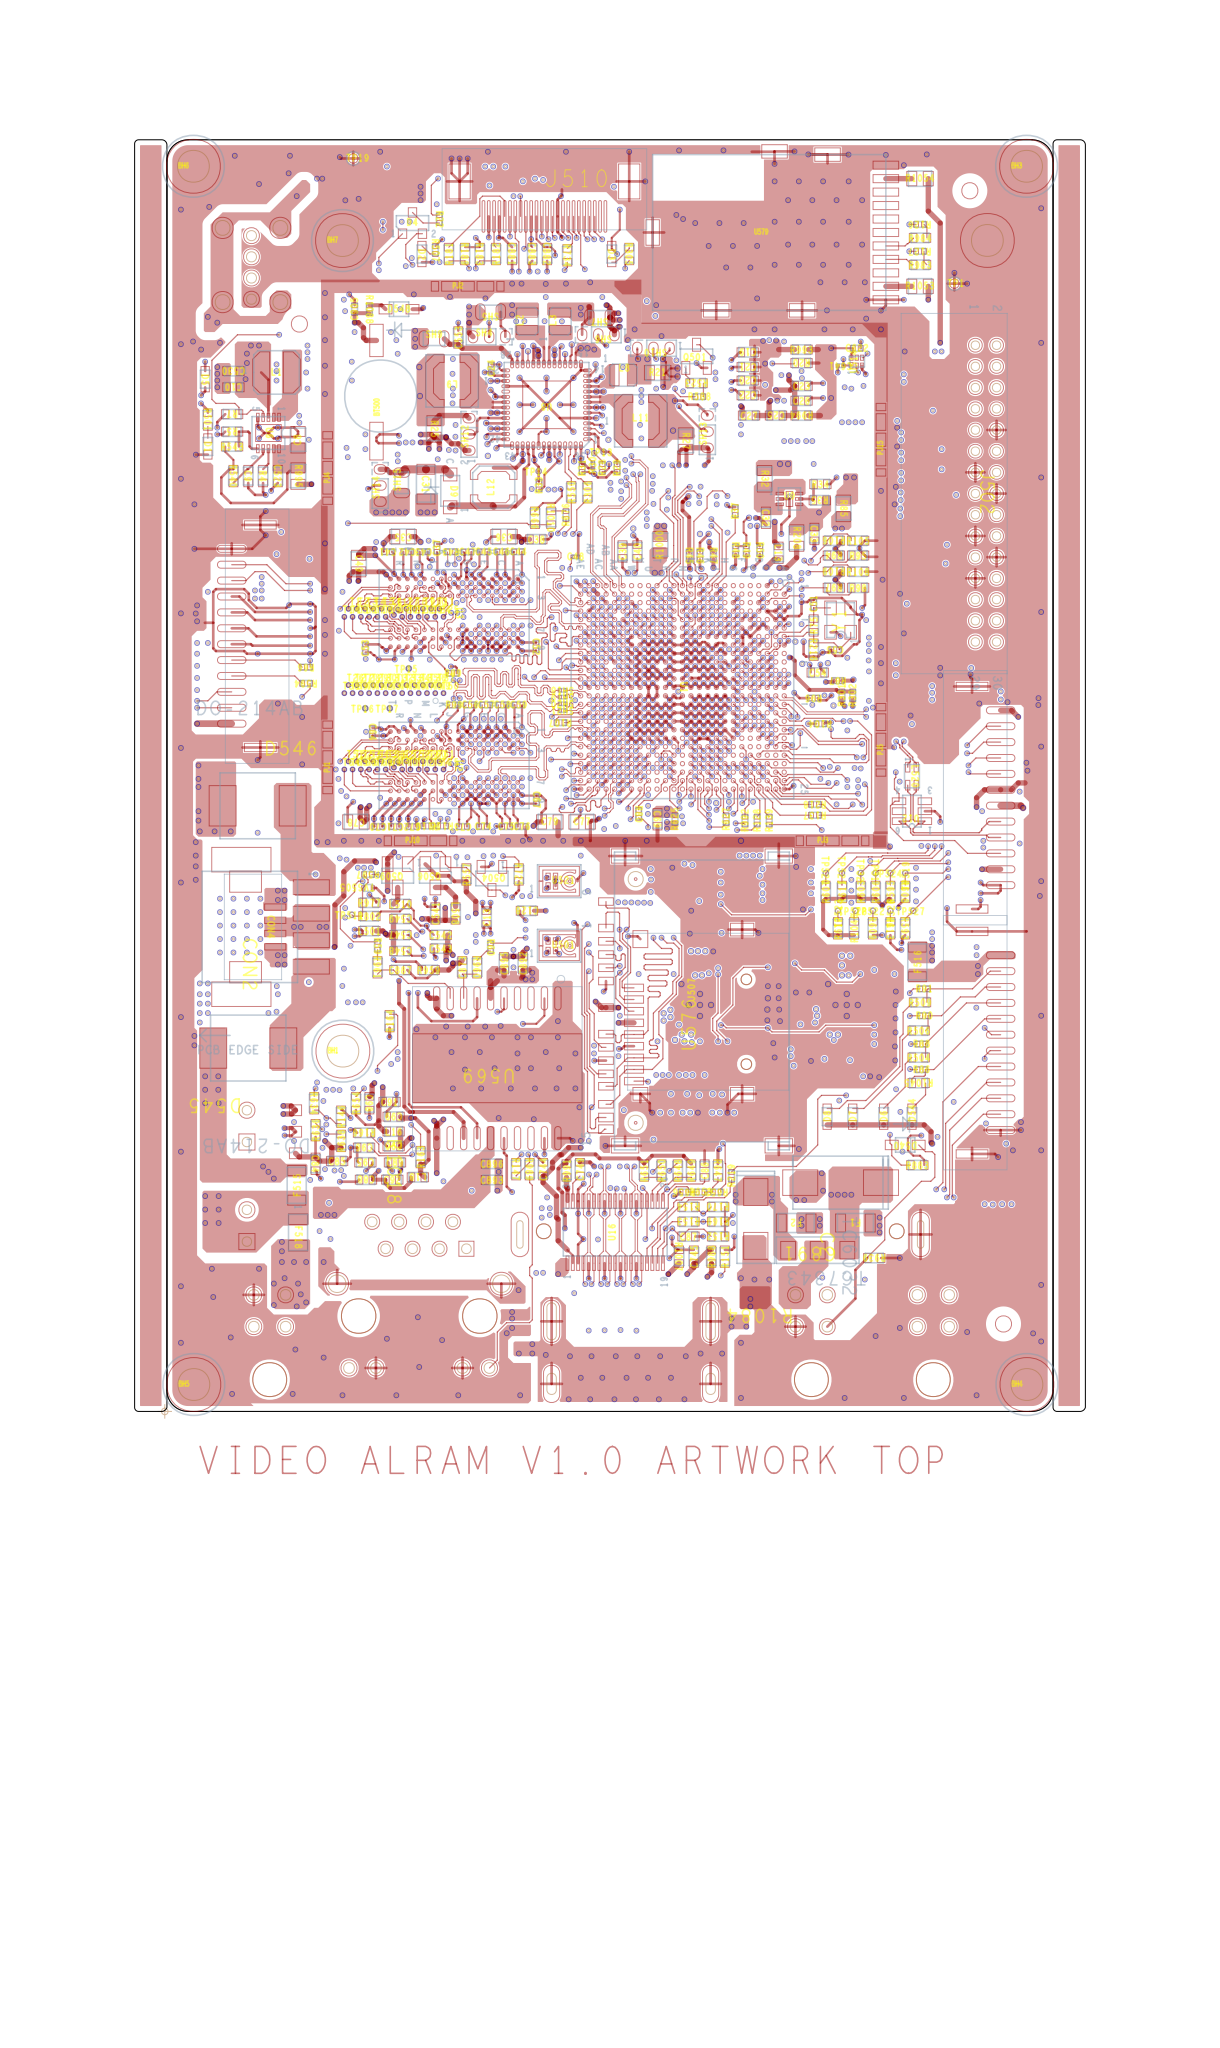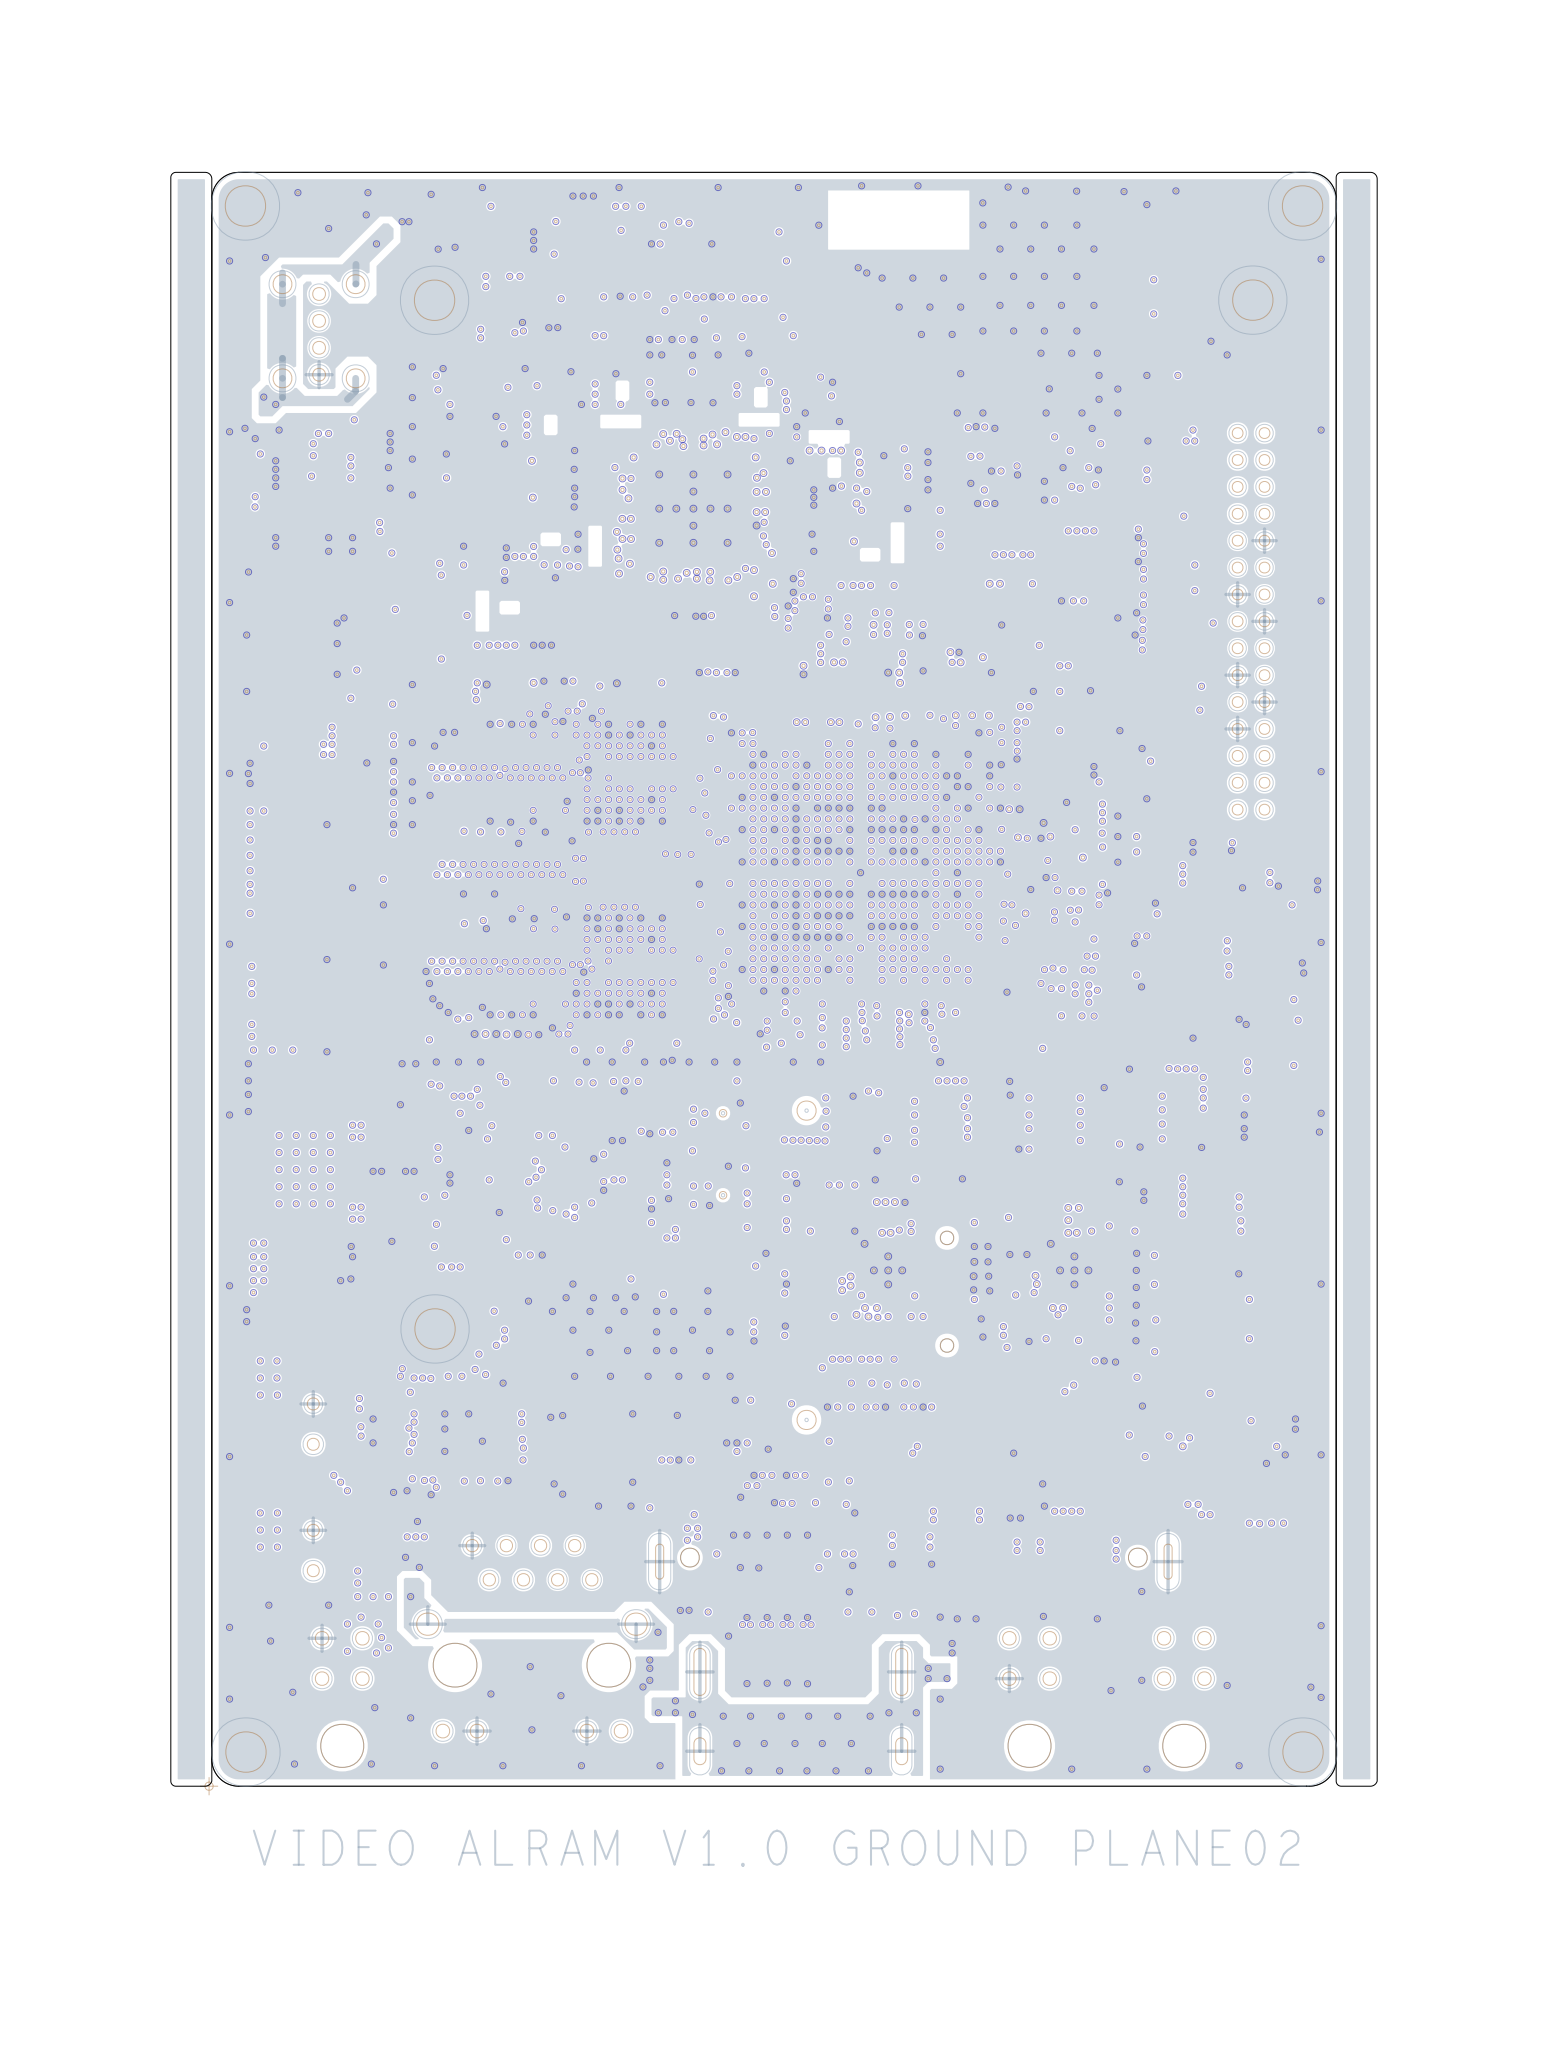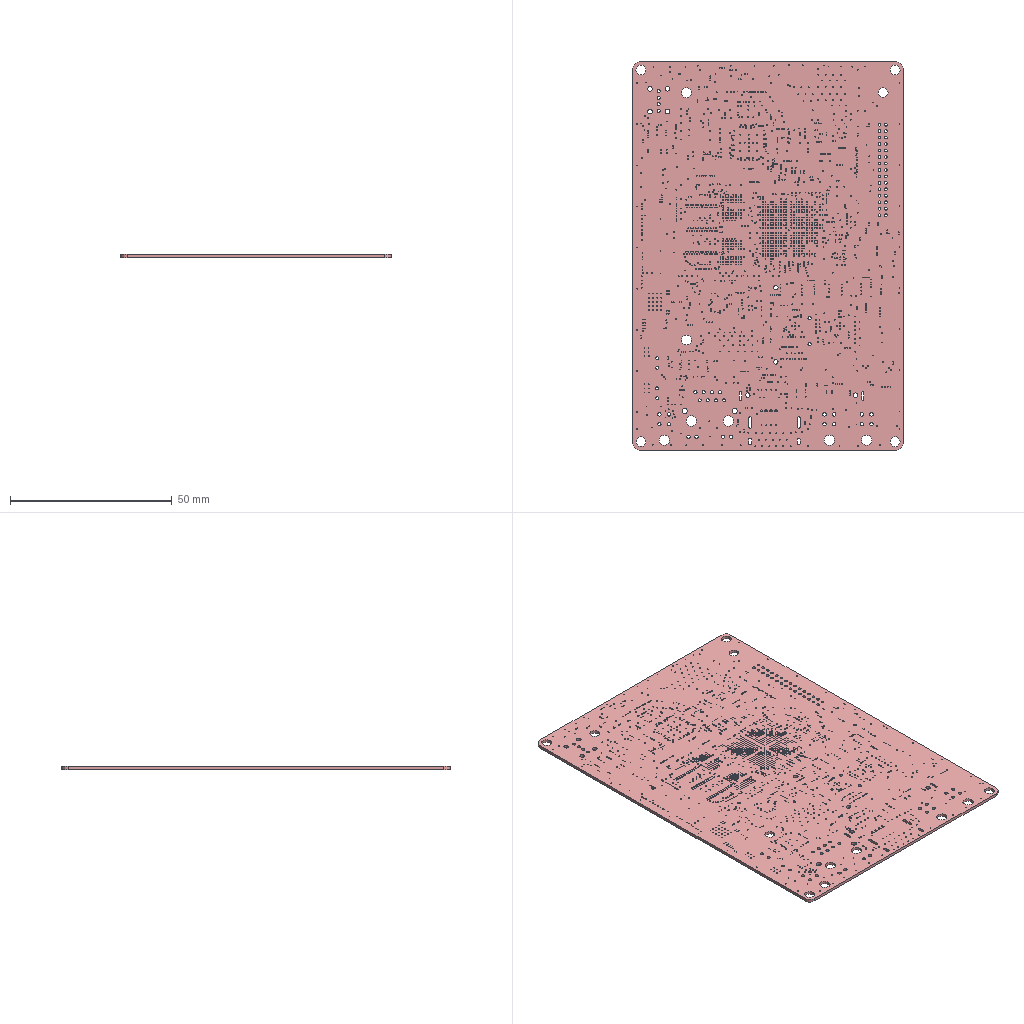Circuit board layout | Cadence Allegro | box 83.6 x 120 x 0.9 mm
Layer stack:
# Cadence Allegro layer stack of  (unit mm; from the constraint file cross-section; dielectric type: 0 not recorded (Allegro does not mark core vs prepreg), 3 surface material)
index,name,kind,layer,copper_thickness_mm,dielectric_type,dielectric_thickness_mm,dielectric_material,dielectric_constant
0,Top Surface,other,,,,,,
1,Dielectric1,dielectric,,,3,0.0127,TAIYO4000_SOLDERMK,4.5
2,TOP,copper,TOP,0.0483,,,,
3,Dielectric2,dielectric,,,0,0.0737,370HR-2GHZ,4.04
4,GND02,copper,GND02,0.0175,,,,
5,Dielectric3,dielectric,,,0,0.1016,370HR-2GHZ,4.04
6,ART03,copper,ART03,0.0175,,,,
7,Dielectric4,dielectric,,,0,0.1397,370HR-2GHZ,4.04
8,POWER04,copper,POWER04,0.0175,,,,
9,Dielectric5,dielectric,,,0,0.2032,FR-4,4.5
10,POWER05,copper,POWER05,0.0175,,,,
11,Dielectric6,dielectric,,,0,0.1397,370HR-2GHZ,4.04
12,ART06,copper,ART06,0.0175,,,,
13,Dielectric7,dielectric,,,0,0.1016,370HR-2GHZ,4.04
14,GND07,copper,GND07,0.0175,,,,
15,Dielectric8,dielectric,,,0,0.0737,370HR-2GHZ,4.04
16,BOTTOM,copper,BOTTOM,0.0483,,,,
17,Dielectric9,dielectric,,,3,0.0127,TAIYO4000_SOLDERMK,4.5
18,Bottom Surface,other,,,,,,
# drill layer pairs: low layer,high layer
drill_pair,TOP,BOTTOM
Part placement, first 503 of 995 lines:
REFDES,COMP_VALUE,SYM_NAME,SYM_X,SYM_Y,SYM_ROTATE,SYM_MIRROR
BH1,SMTSO-M2-2.0ET,HOLE_C5MM_D3MM,661.41,1338.58,0.000,NO
BH2,SMTSO-M2-2.0ET,HOLE_C5MM_D3MM,3055.11,4350.39,0.000,YES
BH3,SMTSO-M2-2.0ET,HOLE_C5MM_D3MM,3200.66,4625.98,0.000,NO
BH4,SMTSO-M2-2.0ET,HOLE_C5MM_D3MM,3202.00,100.00,0.000,NO
BH5,SMTSO-M2-2.0ET,HOLE_C5MM_D3MM,108.00,100.00,0.000,NO
BH6,SMTSO-M2-2.0ET,HOLE_C5MM_D3MM,106.42,4625.98,0.000,NO
BH7,SMTSO-M2-2.0ET,HOLE_C5MM_D3MM,660.00,4350.00,0.000,NO
BT500,BK414,BATT_RETAINER_5P08X5P3,786.26,3791.90,90.000,NO
C1,0.1UF,0603_CC,1520.00,1775.00,180.000,YES
C2,100UF,TC6032,2195.00,715.00,270.000,NO
C3,0.1UF,0603_CC,1640.00,1505.00,270.000,YES
C4,10UF,0603_CC,1640.00,1385.00,90.000,YES
C5,0.01UF,0603_CC,2075.00,1050.00,90.000,YES
C6,0.01UF,0603_CC,2020.00,1050.00,90.000,YES
C7,0.01UF,0603_CC,1965.00,1050.00,90.000,YES
C8,22UF,0805_CC,495.00,3610.00,90.000,NO
C9,0.1UF,0603_CC,310.00,3475.00,270.000,NO
C10,10UF,0603_CC,255.00,3805.00,180.000,NO
C13,0.1UF,0603_CC,1195.00,1835.00,90.000,NO
C15,4.7UF,0603_CC,1157.00,1610.00,90.000,YES
C17,4.7UF,0603_CC,1107.00,1610.00,90.000,YES
C18,2.2uF,0603_CC,1057.00,1610.00,270.000,YES
C19,0.1UF,0603_CC,2165.00,3935.00,180.000,NO
C20,0.1UF,0603_CC,2165.00,3830.00,180.000,NO
C21,0.1UF,0603_CC,2165.00,3880.00,180.000,NO
C22,4.7UF,0603_CC,2165.00,3775.00,180.000,NO
C23,0.1UF,0603_CC,2365.00,3810.00,0.000,NO
C24,0.1UF,0402_CC,1212.65,3875.00,90.000,NO
C25,0.1UF,0603_CC,2270.00,3700.00,180.000,NO
C26,4.7UF,0603_CC,2365.00,3755.00,0.000,NO
C27,0.1UF,0603_CC,2170.00,3700.00,0.000,NO
C31,47uF,1206_CC,970.00,3445.00,270.000,NO
C32,10uF,0603_CC,2232.65,3320.00,270.000,NO
C33,10uF,0603_CC,2412.65,3260.00,270.000,NO
C34,4.7uF,0603_CC,3165.00,2660.00,90.000,YES
C35,22UF,0805_CC,885.00,3250.00,180.000,NO
C36,22UF,0805_CC,1260.00,3250.00,180.000,NO
C37,0.22UF,0402_CC,1010.65,3208.00,90.000,NO
C38,22UF,0603_CC,1380.00,3240.00,0.000,NO
C39,4.7uF,0603_CC,1700.00,3195.00,90.000,NO
C40,22UF,0603_CC,1755.00,3195.00,90.000,NO
C41,0.22UF,0402_CC,828.65,3193.93,180.000,NO
C42,0.22UF,0402_CC,900.65,3193.93,180.000,NO
C43,0.22UF,0402_CC,961.65,3193.93,180.000,NO
C44,0.22UF,0402_CC,1311.65,3193.93,0.000,NO
C45,0.22UF,0402_CC,1183.65,3193.68,0.000,NO
C46,0.22UF,0402_CC,1249.65,3193.68,0.000,NO
C47,0.22UF,0402_CC,1123.91,3193.19,0.000,NO
C48,0.22UF,0201_CC,1525.00,3175.00,0.000,NO
C49,22UF,0805_CC,720.00,3150.00,270.000,NO
C51,18PF,0402_CC,2410.00,3000.00,90.000,NO
C52,0.22UF,0402_CC,1379.05,2841.93,270.000,NO
C53,0.22UF,0402_CC,745.25,2835.00,90.000,NO
C54,22UF,0603_CC,2425.00,2745.00,0.000,NO
C55,18PF,0402_CC,2490.00,2830.00,180.000,NO
C56,0.22UF,0402_CC,1133.65,2625.00,0.000,NO
C57,0.22UF,0402_CC,1193.65,2625.00,0.000,NO
C58,0.22UF,0402_CC,1253.65,2625.00,0.000,NO
C59,0.22UF,0402_CC,1313.65,2625.00,0.000,NO
C61,4.7uF,0603_CC,3010.00,2175.00,270.000,YES
C62,1.0 UF,0603_CC,3065.00,2175.00,270.000,YES
C64,0.22UF,0402_CC,771.25,2525.24,270.000,NO
C66,0.1UF,0603_CC,3145.00,2200.00,0.000,YES
C67,0.22UF,0402_CC,1380.65,2273.00,270.000,NO
C68,22UF,0603_CC,2041.00,2299.00,180.000,YES
C69,22UF,0603_CC,1830.00,2200.00,270.000,NO
C70,0.22UF,0402_CC,792.90,2173.00,180.000,NO
C71,0.22UF,0402_CC,855.90,2173.00,180.000,NO
C72,0.22UF,0402_CC,919.65,2173.00,180.000,NO
C73,0.22UF,0402_CC,1107.65,2173.00,180.000,NO
C74,0.22UF,0402_CC,1181.65,2173.00,0.000,NO
C75,0.22UF,0402_CC,1267.65,2173.00,0.000,NO
C76,0.22UF,0402_CC,1325.65,2173.00,0.000,NO
C77,22UF,0805_CC,1550.00,2190.00,0.000,NO
C78,22UF,0805_CC,710.00,2190.00,180.000,NO
C79,22UF,0805_CC,1430.00,2190.00,0.000,NO
C83,0.1UF,0603_CC,2755.00,2130.00,0.000,YES
C84,1.0 UF,0603_CC,560.00,920.00,270.000,NO
C85,0.1UF,0603_CC,640.00,930.00,0.000,NO
C86,0.1UF,0603_CC,2005.00,895.00,90.000,NO
C87,0.1UF,0603_CC,1945.00,650.00,0.000,NO
C88,1.0 UF,0603_CC,747.20,861.00,180.000,NO
C89,0.1UF,0603_CC,855.00,925.00,0.000,NO
C90,0.1UF,0603_CC,850.00,985.00,180.000,NO
C91,10UF,0603_CC,835.00,1150.00,0.000,NO
C92,0.1UF,0603_CC,845.00,861.00,0.000,NO
C93,0.1UF,0603_CC,935.00,1355.00,270.000,YES
C94,0.22UF,0603_CC,1855.00,4080.00,270.000,YES
C95,0.1UF,0603_CC,745.00,925.00,180.000,NO
C96,1.0 UF,0603_CC,740.00,980.00,180.000,NO
C97,10UF,0603_CC,980.00,1110.00,180.000,YES
C98,0.1UF,0603_CC,760.00,1145.00,270.000,NO
C99,0.1UF,0603_CC,850.00,1095.00,180.000,NO
C128,0.1UF,0603_CC,1345.00,1860.00,180.000,NO
C501,100uF,1206_CC,445.00,3930.00,180.000,YES
C504,2.2uF,0603_CC,1600.00,3255.00,0.000,YES
C505,10UF,0603_CC,470.00,3800.00,180.000,YES
C506,1.0 UF,0603_CC,470.00,3855.00,180.000,YES
C507,10UF,0603_CC,1899.89,1720.00,0.000,YES
C508,10UF,0603_CC,2454.89,1710.00,0.000,YES
C510,1.0 UF,0603_CC,1899.89,1665.00,0.000,YES
C511,1.0 UF,0603_CC,2454.89,1655.00,0.000,YES
C512,0.1UF,0603_CC,1805.00,1665.00,180.000,YES
C513,0.1UF,0603_CC,2375.00,1670.00,90.000,YES
C514,1.0 UF,0603_CC,2180.00,1705.00,270.000,YES
C515,1.0 UF,0603_CC,2710.00,1535.00,180.000,YES
C517,0.15UF,0603_CC,2160.00,1525.00,180.000,YES
C518,0.15UF,0603_CC,2710.00,1485.00,180.000,YES
C520,10UF,0603_CC,1797.89,1468.00,0.000,YES
C521,10UF,0603_CC,2364.89,1470.00,0.000,YES
C523,0.1UF,0603_CC,420.00,3475.00,270.000,NO
C526,10UF,0603_CC,1830.00,1345.00,0.000,YES
C527,10UF,0603_CC,2420.00,1305.00,90.000,YES
C528,4.7uF,0603_CC,2255.00,1285.00,180.000,YES
C529,4.7uF,0603_CC,2710.00,1280.00,180.000,YES
C530,0.1UF,0603_CC,255.00,3865.00,180.000,NO
C539,4.7UF,0603_CC,1195.00,1835.00,270.000,YES
C540,1.0UF,0603_CC,1235.00,1640.00,180.000,YES
C541,4.7uF,0603_CC,1005.00,1850.00,90.000,NO
C542,4.7UF,0603_CC,1025.00,1770.00,0.000,NO
C543,2.2uF,0603_CC,1025.00,1720.00,0.000,NO
C544,22UF,0603_CC,1325.00,4120.00,270.000,YES
C545,22UF,0603_CC,1250.00,4120.00,270.000,YES
C546,22UF,0603_CC,1510.00,4120.00,270.000,YES
C547,2.2uF,0603_CC,875.00,1770.00,180.000,NO
C548,2.2uF,0603_CC,875.00,1710.00,180.000,NO
C549,1.0 UF,0603_CC,875.00,1830.00,180.000,NO
C550,4.7uF,0603_CC,1510.00,4025.00,270.000,YES
C551,4.7uF,0603_CC,1445.00,4025.00,270.000,YES
C552,4.7uF,0603_CC,1372.65,4025.00,270.000,YES
C553,4.7uF,0603_CC,1090.00,3990.00,90.000,NO
C554,4.7uF,0603_CC,1275.00,4000.00,270.000,YES
C555,22UF,0603_CC,1580.00,4120.00,270.000,YES
C556,4.7uF,0603_CC,1560.00,3890.00,90.000,YES
C557,2.2uF,0603_CC,2803.00,3938.00,0.000,YES
C558,0.1UF,0603_CC,1485.00,2020.00,180.000,YES
C559,22UF,0603_CC,1702.65,3915.00,0.000,YES
C560,22UF,0603_CC,1005.00,3910.00,180.000,YES
C561,0.47uF,0402_CC,1505.00,3885.00,90.000,YES
C562,0.47uF,0402_CC,1317.65,3885.00,90.000,YES
C563,0.1UF,0402_CC,1447.65,3885.00,90.000,YES
C564,0.1UF,0402_CC,1387.65,3885.00,90.000,YES
C565,0.1UF,0402_CC,1257.07,3861.73,180.000,YES
C566,22UF,0603_CC,1005.00,3855.00,180.000,YES
C567,22UF,0603_CC,1792.65,3850.00,90.000,YES
C568,4.7uF,0603_CC,1701.65,3846.00,180.000,YES
C569,0.1UF,0402_CC,1555.00,3825.00,0.000,YES
C570,1.0UF,0402_CC,1280.00,3815.00,180.000,YES
C571,22UF,0603_CC,1005.00,3800.00,180.000,YES
C572,4.7uF,0603_CC,1140.00,3785.00,0.000,YES
C573,4.7uF,0603_CC,1700.00,3780.00,180.000,YES
C574,22UF,0603_CC,1832.65,3770.00,0.000,YES
C575,0.1UF,0402_CC,1280.00,3770.00,180.000,YES
C576,0.1UF,0402_CC,1555.00,3780.00,0.000,YES
C577,22UF,0603_CC,1005.00,3745.00,180.000,YES
C578,4.7uF,0603_CC,1700.00,3720.00,180.000,YES
C579,0.1UF,0402_CC,1555.00,3725.00,0.000,YES
C580,4.7uF,0603_CC,1137.65,3725.00,0.000,YES
C581,22UF,0603_CC,1832.65,3720.00,0.000,YES
C582,0.1UF,0402_CC,1280.00,3710.00,180.000,YES
C583,22UF,0603_CC,1832.65,3665.00,0.000,YES
C584,4.7uF,0603_CC,1137.65,3665.00,0.000,YES
C586,0.47uF,0402_CC,1280.00,3660.00,180.000,YES
C589,10uF,0603_CC,1380.65,3620.00,270.000,YES
C590,0.1UF,0402_CC,1280.00,3620.00,180.000,YES
C591,22UF,0603_CC,1832.65,3610.00,0.000,YES
C592,1.0UF,0402_CC,1430.00,3600.00,270.000,YES
C593,0.1UF,0402_CC,1330.00,3600.00,270.000,YES
C594,0.22UF,0402_CC,1475.00,3600.00,270.000,YES
C595,4.7uF,0603_CC,1135.00,3610.00,0.000,YES
C596,0.47uF,0402_CC,1280.00,3580.00,180.000,YES
C597,0.1UF,0402_CC,1525.00,3600.00,270.000,YES
C599,1.0UF,0402_CC,1422.65,3470.00,90.000,YES
C600,1.0UF,0402_CC,1462.65,3469.74,90.000,YES
C601,10uF,0603_CC,1330.00,3455.00,90.000,YES
C603,0.1UF,0603_CC,2775.00,2865.00,270.000,YES
C604,22UF,0603_CC,1755.00,3195.00,270.000,YES
C605,22UF,0603_CC,2280.00,3200.00,270.000,YES
C606,4.7UF,0603_CC,2230.00,3200.00,270.000,YES
C607,4.7UF,0603_CC,2180.00,3200.00,270.000,YES
C608,4.7UF,0603_CC,2130.00,3200.00,270.000,YES
C609,4.7UF,0603_CC,2080.00,3200.00,270.000,YES
C610,4.7UF,0603_CC,1987.65,3190.00,270.000,YES
C611,22UF,0603_CC,1860.00,3195.00,270.000,YES
C612,22UF,0603_CC,1810.00,3195.00,270.000,YES
C613,0.22UF,0402_CC,900.65,3194.00,0.000,YES
C614,0.22UF,0402_CC,837.15,3194.00,0.000,YES
C615,0.22UF,0402_CC,1262.65,3193.93,180.000,YES
C616,0.22UF,0402_CC,1200.65,3193.93,0.000,YES
C617,0.22UF,0402_CC,1108.65,3193.93,180.000,YES
C618,0.22UF,0402_CC,962.65,3193.93,180.000,YES
C619,0.22UF,0201_CC,1530.00,3125.00,90.000,YES
C620,0.22UF,0402_CC,1405.00,3095.00,270.000,YES
C621,0.1UF,0402_CC,1625.00,3055.00,90.000,YES
C622,0.22UF,0402_CC,2570.00,3950.00,0.000,NO
C623,22UF,0603_CC,2360.00,2960.00,0.000,YES
C624,18PF,0402_CC,2525.00,2995.00,180.000,YES
C625,0.22UF,0201_CC,1969.89,2925.00,270.000,YES
C626,0.22UF,0201_CC,2160.00,2915.00,180.000,YES
C627,10UF,0603_CC,2370.00,2890.00,180.000,YES
C628,0.22UF,0201_CC,2197.65,2895.00,270.000,YES
C629,0.22UF,0201_CC,1918.65,2894.00,90.000,YES
C630,0.22UF,0201_CC,1894.80,2894.00,90.000,YES
C632,0.22UF,0201_CC,1750.00,2865.00,90.000,YES
C633,0.22UF,0201_CC,2170.65,2863.50,270.000,YES
C634,0.22UF,0201_CC,2148.65,2863.50,270.000,YES
C635,0.22UF,0201_CC,2085.15,2862.50,90.000,YES
C636,0.22UF,0201_CC,2062.65,2862.50,90.000,YES
C637,0.22UF,0201_CC,2034.65,2862.50,90.000,YES
C638,0.22UF,0201_CC,2009.65,2862.50,90.000,YES
C639,18PF,0402_CC,2455.00,2875.00,180.000,YES
C640,0.22UF,0201_CC,2107.15,2857.50,90.000,YES
C641,0.22UF,0201_CC,2510.00,3885.00,180.000,NO
C642,0.22UF,0201_CC,2220.00,2840.00,180.000,YES
C643,0.22UF,0201_CC,1985.64,2847.48,270.000,YES
C644,0.22UF,0201_CC,1859.66,2847.48,270.000,YES
C645,0.22UF,0201_CC,1828.16,2847.48,270.000,YES
C646,0.22UF,0201_CC,1796.67,2847.48,270.000,YES
C647,0.22UF,0402_CC,1400.00,2820.00,90.000,YES
C648,0.22UF,0402_CC,2467.65,2825.00,270.000,YES
C649,22UF,0603_CC,1907.15,2824.50,90.000,YES
C650,0.22UF,0201_CC,1733.67,2815.99,0.000,YES
C651,0.22UF,0201_CC,2287.65,2810.00,90.000,YES
C652,0.22UF,0201_CC,2097.65,2810.00,180.000,YES
C653,0.22UF,0402_CC,745.25,2835.00,270.000,YES
C654,22UF,0603_CC,2387.65,2807.00,180.000,YES
C655,0.01UF,0201_CC,2096.88,2788.50,180.000,YES
C656,0.22UF,0201_CC,1796.67,2785.49,90.000,YES
C657,0.22UF,0201_CC,2138.85,2784.50,270.000,YES
C658,0.22UF,0201_CC,2048.63,2784.49,270.000,YES
C659,0.22UF,0201_CC,2017.14,2784.49,270.000,YES
C660,0.22UF,0201_CC,1985.64,2784.49,270.000,YES
C661,0.22UF,0201_CC,1828.16,2784.49,90.000,YES
C662,0.22UF,0201_CC,1733.67,2784.49,0.000,YES
C663,0.22UF,0201_CC,1858.70,2762.02,90.000,YES
C664,0.22UF,0201_CC,1772.70,2753.00,180.000,YES
C665,0.22UF,0201_CC,1729.67,2752.99,0.000,YES
C666,0.22UF,0402_CC,867.90,2744.93,180.000,YES
C667,0.22UF,0201_CC,1957.65,2736.50,90.000,YES
C668,0.22UF,0201_CC,2091.00,2735.00,0.000,YES
C669,22UF,0603_CC,1907.15,2730.50,90.000,YES
C670,0.22UF,0201_CC,2048.63,2727.26,270.000,YES
C671,0.22UF,0201_CC,2017.14,2727.26,270.000,YES
C672,0.22UF,0201_CC,1985.64,2727.26,270.000,YES
C673,4.7UF,0603_CC,2392.65,2725.00,0.000,YES
C674,0.22UF,0201_CC,1828.16,2721.50,270.000,YES
C675,0.22UF,0201_CC,1733.67,2721.50,0.000,YES
C676,0.22UF,0201_CC,1796.67,2720.50,270.000,YES
C677,0.22UF,0201_CC,1859.70,2718.50,270.000,YES
C678,0.22UF,0201_CC,2159.65,2685.00,180.000,YES
C679,22UF,0603_CC,1978.65,2675.26,0.000,YES
C680,22UF,0603_CC,2070.15,2675.16,180.000,YES
C681,4.7UF,0603_CC,2392.65,2675.00,180.000,YES
C682,22UF,0603_CC,1835.65,2674.25,180.000,YES
C683,22UF,0603_CC,1744.65,2674.25,0.000,YES
C684,0.22UF,0201_CC,2159.65,2664.00,180.000,YES
C685,0.22UF,0201_CC,2080.13,2630.13,90.000,YES
C686,0.22UF,0201_CC,2048.63,2630.13,90.000,YES
C687,0.22UF,0201_CC,2017.14,2630.13,90.000,YES
C688,0.22UF,0201_CC,1985.64,2630.13,90.000,YES
C689,0.22UF,0201_CC,1954.15,2630.13,90.000,YES
C690,0.22UF,0201_CC,1859.66,2627.01,90.000,YES
C691,0.22UF,0201_CC,1828.16,2627.01,90.000,YES
C692,0.22UF,0201_CC,1796.67,2627.01,90.000,YES
C693,0.22UF,0201_CC,2160.00,2610.00,180.000,YES
C694,22UF,0603_CC,1907.15,2620.50,270.000,YES
C695,0.22UF,0201_CC,2108.63,2587.10,270.000,YES
C696,0.22UF,0201_CC,1733.67,2595.51,0.000,YES
C698,0.22UF,0201_CC,2080.13,2587.10,270.000,YES
C701,0.22UF,0201_CC,2048.63,2587.10,270.000,YES
C702,0.22UF,0201_CC,2017.14,2587.10,270.000,YES
C703,0.22UF,0201_CC,1985.64,2587.10,270.000,YES
C704,0.22UF,0201_CC,1954.15,2587.10,270.000,YES
C705,0.22UF,0201_CC,1859.66,2564.02,90.000,YES
C706,0.22UF,0201_CC,1828.16,2564.02,90.000,YES
C707,0.22UF,0201_CC,1796.67,2564.02,90.000,YES
C708,0.22UF,0201_CC,1733.67,2564.02,0.000,YES
C709,0.22UF,0201_CC,2105.65,2538.00,90.000,YES
C710,0.22UF,0201_CC,2080.13,2537.52,90.000,YES
C711,0.22UF,0201_CC,2048.63,2537.52,90.000,YES
C712,0.22UF,0201_CC,2017.14,2537.52,90.000,YES
C713,0.22UF,0201_CC,1985.64,2537.52,90.000,YES
C714,0.22UF,0201_CC,1954.15,2537.52,90.000,YES
C715,0.22UF,0201_CC,1733.67,2532.52,0.000,YES
C716,22UF,0603_CC,1907.15,2530.50,90.000,YES
C717,0.22UF,0402_CC,740.00,2550.00,180.000,YES
C718,0.22UF,0402_CC,1400.00,2510.00,270.000,YES
C719,0.22UF,0201_CC,1868.65,2516.00,270.000,YES
C720,0.22UF,0201_CC,1828.16,2501.02,90.000,YES
C721,0.22UF,0201_CC,1796.67,2501.02,90.000,YES
C722,0.22UF,0201_CC,1765.17,2501.02,90.000,YES
C723,0.22UF,0201_CC,2127.70,2496.05,0.000,YES
C724,0.22UF,0201_CC,1985.64,2494.50,270.000,YES
C725,0.22UF,0201_CC,1906.70,2473.55,180.000,YES
C726,1.0UF,0402_CC,1875.00,2325.00,0.000,YES
C727,0.22UF,0201_CC,1581.70,2203.05,90.000,YES
C728,0.22UF,0201_CC,1556.70,2203.05,90.000,YES
C729,22UF,0603_CC,1760.00,2200.00,90.000,YES
C730,22UF,0603_CC,1830.00,2200.00,90.000,YES
C731,0.22UF,0402_CC,1325.65,2173.00,180.000,YES
C732,0.22UF,0402_CC,1267.65,2173.00,180.000,YES
C733,0.22UF,0402_CC,1182.15,2173.00,180.000,YES
C734,0.22UF,0402_CC,1108.15,2173.00,180.000,YES
C735,0.22UF,0402_CC,855.90,2173.00,0.000,YES
C736,0.22UF,0402_CC,792.90,2173.00,0.000,YES
C737,0.22UF,0402_CC,1030.00,2175.00,0.000,YES
C738,0.1UF,0603_CC,2140.00,370.00,90.000,YES
C739,470PF,0603_CC,1400.00,1060.00,270.000,YES
C740,470PF,0603_CC,1465.00,1060.00,90.000,YES
C741,470PF,0603_CC,610.00,835.00,90.000,YES
C742,0.1UF,0603_CC,1505.00,475.00,180.000,YES
C743,4.7uF,0603_CC,1405.00,475.00,0.000,YES
C744,0.1UF,0603_CC,1405.00,899.90,90.000,NO
C745,0.1UF,0603_CC,1965.00,575.00,90.000,NO
C746,0.22UF,0603_CC,1850.00,3965.00,180.000,YES
C748,22PF,0603_CC,980.00,1030.00,270.000,YES
C749,0.1UF,0603_CC,1542.00,900.00,90.000,NO
C750,22PF,0603_CC,980.00,930.00,90.000,YES
C753,0.22UF,0603_CC,925.00,4095.00,270.000,YES
C754,0.22UF,0603_CC,895.00,3955.00,90.000,YES
C755,0.1UF,0603_CC,760.00,4050.00,0.000,YES
C758,1000PF,0603_CC,835.00,3550.00,90.000,YES
C759,56PF,0603_CC,710.00,3655.00,90.000,YES
C760,56PF,0603_CC,780.00,3655.00,90.000,YES
C761,10UF,0603_CC,3160.00,1155.00,90.000,YES
C763,0.1UF,0603_CC,3100.00,1155.00,90.000,YES
C788,10UF,0603_CC,720.00,4565.00,90.000,YES
C820,1.0 UF,0603_CC,3135.00,710.00,270.000,YES
C862,0.22UF,0603_CC,955.00,1610.00,90.000,YES
C863,0.22UF,0603_CC,905.00,1610.00,90.000,YES
C867,1.0 UF,0603_CC,165.00,1420.00,90.000,YES
C868,1.0 UF,0603_CC,235.00,1420.00,90.000,YES
C870,1.0 UF,0603_CC,410.00,2970.00,270.000,YES
C871,220UF,CAPDIP0903,305.00,690.00,270.000,YES
C873,1uF,0603_CC,1105.00,1650.00,90.000,NO
C881,10UF,0603_CC,1290.00,4300.00,270.000,NO
C882,10UF,0603_CC,1420.00,4300.00,270.000,NO
C883,10UF,0603_CC,1365.00,4300.00,270.000,NO
C887,10uF,0603_CC,875.00,1640.00,0.000,NO
C888,0.1UF,0603_CC,645.00,4530.00,180.000,YES
C889,0.1UF,0603_CC,550.00,4550.00,180.000,YES
C890,0.01UF,0603_CC,1910.00,1050.00,90.000,YES
C891,100UF,TC7343,2510.00,850.00,180.000,NO
C892,0.1UF,0603_CC,1330.00,1665.00,90.000,NO
C893,1.0 UF,0603_CC,1215.00,860.00,0.000,NO
C894,220UF,CAPDIP0903,305.00,1060.00,270.000,YES
C895,0.1UF,0603_CC,1260.00,1665.00,90.000,NO
C896,0.1UF,0603_CC,1215.00,920.00,0.000,NO
C897,0.1UF,0603_CC,1330.00,390.00,270.000,YES
C898,0.1UF,0603_CC,3130.00,2570.00,270.000,YES
C899,0.1UF,0603_CC,3025.00,2570.00,270.000,YES
C900,0.1UF,0603_CC,3080.00,2570.00,270.000,YES
C901,0.1UF,0603_CC,3162.07,2458.64,90.000,YES
C903,0.1UF,0603_CC,2820.00,2564.41,270.000,YES
C905,1.0UF,0402_CC,705.00,4095.00,90.000,NO
CON2,CON_1X4,BATTERY,300.00,1800.00,270.000,NO
CON4,CON_1X4,CON_TB_4F_2P5_9X10P5,375.00,1800.00,270.000,NO
D1,LED_GREEN,LED_0603,160.00,3585.00,270.000,NO
D2,LED_GREEN,LED_0603,955.00,4300.00,270.000,NO
D3,RED,LED_0603,1660.00,4300.00,270.000,NO
D4,BAT54CLT1,SOT23_A,920.00,4415.00,0.000,NO
D5,RED,LED_0603,150.00,3835.00,270.000,NO
D6,LED_GREEN,LED_0603,2670.00,1095.00,90.000,NO
D7,LED_GREEN,LED_0603,2555.00,1095.00,90.000,NO
D8,LED_GREEN,LED_0603,2460.00,1095.00,90.000,NO
D9,MBR140SFT,SOD123LF,1060.00,3420.00,270.000,NO
D10,NSR0320,SOD323,2455.00,3100.00,180.000,YES
D500,RB521CS-30,DO_VMN2,400.00,3230.00,270.000,YES
D501,ESD9L5.0ST5G,SOD-923,160.00,3370.00,180.000,YES
D502,SMLJ60S6,DO214AB_SM,260.00,3600.00,180.000,YES
D503,MMSZ5231BT1G,SOD123,485.00,3020.00,90.000,YES
D504,BAT54HT1,SOD323,1900.00,1145.00,270.000,YES
D539,SS54,DO-214AB,315.00,2050.00,180.000,YES
D540,NSR0320,SOD323,2750.00,990.00,90.000,NO
D541,LED_ORANGE,LED_0603,1635.00,1065.00,90.000,YES
D544,LED_GREEN,LED_0603,2775.00,1095.00,90.000,NO
D545,SS54,DO-214AB,310.00,1350.00,180.000,NO
D546,SS54,DO-214AB,345.00,2250.00,0.000,NO
D547,SS54,DO-214AB,315.00,2750.00,180.000,YES
D548,NSR0320,SOD323,870.00,4095.00,270.000,NO
F1,1A/32V,1206_CC,2565.00,700.00,180.000,NO
F2,1A/32V,1206_CC,2345.00,700.00,180.000,NO
F500,5A/32V,FUSE_3P4X1P8,300.00,2950.00,0.000,YES
F513,1A/32V,1206_CC,2220.00,1070.00,90.000,YES
F514,1A/32V,1206_CC,2315.00,1070.00,90.000,YES
F515,1A/32V,1206_CC,490.00,840.00,90.000,NO
F516,1A/32V,1206_CC,2795.00,1670.00,90.000,NO
F518,5A/32V,FUSE_3P4X1P8,495.00,665.00,270.000,NO
J7,HR911105A,HR911105A,945.07,344.49,0.000,YES
J8,10029449-001RLF,HDMI,1732.00,-78.74,0.000,YES
J502,CON 30,CON_2X15_2_0,3050.00,3410.00,270.000,NO
J507,CONN CRD 19,CON19_SDCARD_28X16_SM,1995.00,1525.00,90.000,NO
J510,FPC-24-0.5,OV5642,1410.00,4550.00,0.000,NO
J524,MICRO USB AB 5,USB_A-RECEPT-R_A-DIP_1,322.00,4368.30,180.000,YES
J552,CON5,CON5,2854.33,314.96,270.000,YES
J553,CON5,CON5,2401.56,314.96,270.000,YES
J559,HDR12,HDR12,3128.11,1370.00,270.000,NO
J560,HDR12,HDR12,3128.11,2280.00,270.000,NO
J561,HDR12,HDR12,225.00,2880.00,90.000,NO
J562,CON5,CON5,389.76,314.96,270.000,YES
L1,1.2uH,IND_VLCF4018,415.00,3860.00,0.000,NO
L2,1UH,IND_VLS252010,1346.08,4050.07,90.000,NO
L3,1UH,IND_VLS252010,1468.06,4050.07,90.000,NO
L4,100 OHM@100MHZ,0603_CC,875.00,1770.00,0.000,YES
L5,100 OHM@100MHZ,0603_CC,875.00,1830.00,0.000,YES
L6,100 OHM@100MHZ,0603_CC,875.00,1880.00,0.000,YES
L7,100 OHM@100MHZ,0603_CC,885.00,1990.00,270.000,YES
L8,1UH,IND_VLS252010,1702.65,3850.00,0.000,NO
L9,1uH,IND_5015,1066.98,3828.43,180.000,NO
L11,1uH,IND_5015,1767.65,3680.00,0.000,NO
L12,2.2uH,IND_LPS4018,1221.65,3434.00,90.000,NO
L13,120OHM,0603_CC,2280.00,3190.00,270.000,NO
L15,470OHM,0603_CC,3145.00,2150.00,180.000,YES
L16,120OHM,0603_CC,850.00,1040.00,0.000,NO
L18,120OHM,0603_CC,940.00,870.00,180.000,NO
L19,4.7UH,IND_VLS3012_SM,975.00,1210.00,270.000,YES
L501,120OHM,0603_CC,760.00,1785.00,0.000,NO
L502,1UH,IND_VLS252010,1820.30,1556.92,90.000,YES
L503,1UH,IND_VLS252010,2365.30,1556.92,90.000,YES
L506,120OHM,0603_CC,1235.00,1590.00,0.000,YES
L507,100 OHM@100MHZ,0603_CC,3060.00,610.00,90.000,YES
L508,120OHM,0603_CC,1080.00,1850.00,270.000,NO
L509,100 OHM@100MHZ,0603_CC,3135.00,610.00,90.000,YES
L510,120OHM,0603_CC,875.00,1885.00,0.000,NO
L511,90OHM,IND4_CHOKE_0805,2803.00,3623.00,180.000,YES
L512,90OHM,IND4_CHOKE_0805,2803.00,3548.00,180.000,YES
L513,90OHM,IND4_CHOKE_0805,2803.00,3473.00,180.000,YES
L514,90OHM,IND4_CHOKE_0805,2805.00,3400.00,180.000,YES
L519,470OHM,0603_CC,3162.00,2355.00,90.000,YES
L520,90OHM,IND4_CHOKE_0805,2775.00,2360.00,270.000,NO
L523,470OHM,0603_CC,645.00,4590.00,0.000,YES
L544,47UH/5A,MT105,310.00,2400.00,270.000,YES
L546,90OHM,IND4_CHOKE_0805,2805.00,3325.00,180.000,YES
PJ1,PTC0703B,PTC0703B_SMD,605.00,2430.00,90.000,NO
PJ2,PTC0703B,PTC0703B_SMD,1125.00,4180.00,0.000,NO
PJ3,PTC0703B,PTC0703B_SMD,2480.00,2120.00,0.000,NO
PJ4,PTC0703B,PTC0703B_SMD,605.00,3505.00,90.000,NO
PJ5,PTC0703B,PTC0703B_SMD,2660.00,2495.00,90.000,NO
PJ6,PTC0703B,PTC0703B_SMD,2405.00,2120.00,0.000,YES
PJ7,PTC0703B,PTC0703B_SMD,950.00,2120.00,0.000,YES
PJ8,PTC0703B,PTC0703B_SMD,995.00,4195.00,0.000,YES
PJ9,PTC0703B,PTC0703B_SMD,2275.00,4195.00,0.000,YES
PJ10,PTC0703B,PTC0703B_SMD,950.00,2120.00,0.000,NO
PJ11,PTC0703B,PTC0703B_SMD,585.00,3615.00,90.000,YES
PJ12,PTC0703B,PTC0703B_SMD,585.00,2660.00,90.000,YES
PJ13,PTC0703B,PTC0703B_SMD,2660.00,3845.00,90.000,YES
PJ14,PTC0703B,PTC0703B_SMD,2660.00,2310.00,90.000,YES
PJ15,PTC0703B,PTC0703B_SMD,2660.00,3610.00,90.000,NO
Q1,MBT3906DW1T1,SOT363,480.00,3230.00,0.000,YES
Q6,FDMS6681Z,SO8_PAK,250.00,3200.00,270.000,YES
Q501,MMBT3904LT1G,SOT23,1975.00,3920.00,0.000,NO
Q503,NTS4001NT1G,SC70_3,480.00,3590.00,0.000,YES
Q504,2N7002,SOT23,1215.00,1980.00,180.000,NO
Q505,IRLML6401,SOT-23,1290.00,1830.00,180.000,YES
Q506,IRLML6401,SOT-23,1005.00,1990.00,180.000,NO
Q509,IRLML6401,SOT-23,865.00,1990.00,180.000,NO
Q510,2N7002,SOT23,1012.65,3463.00,270.000,YES
Q511,IRLML6401,SOT-23,1220.00,3455.00,270.000,YES
Q512,BSS138DW-7,SC70-6,1340.08,4434.93,0.000,YES
Q513,IRLML6401,SOT-23,2945.00,980.00,90.000,YES
Q514,IRLML6401,SOT-23,1625.00,4585.00,270.000,YES
Q515,2N7002,SOT23,1545.00,4445.00,0.000,YES
Q535,MMBT3904LT1G,SOT23,2730.00,1070.00,180.000,YES
Q539,MMBT3904LT1G,SOT23,585.00,1715.00,0.000,YES
QZ500,32.768KHZ,XTAL2-3P2X1P5-SM,2537.65,2890.00,90.000,YES
R1,10.0K,0603_CC,490.00,3340.00,90.000,YES
R2,10.0K,0603_CC,490.00,3450.00,90.000,YES
R3,10.0K,0603_CC,470.00,3140.00,0.000,YES
R4,0,0603_CC,365.00,3475.00,270.000,NO
R5,0,0603_CC,250.00,3640.00,180.000,NO
R7,4.7K,0603_CC,250.00,3705.00,180.000,NO
R10,22,0603_CC,1234.00,1694.00,0.000,YES
R11,0,0603_CC,1245.00,1980.00,90.000,YES
R12,0,0603_CC,1185.00,1980.00,90.000,YES
R13,0,0603_CC,1125.00,1980.00,90.000,YES
R14,22,0603_CC,1065.00,1980.00,90.000,YES
R16,0,0603_CC,1005.00,1980.00,90.000,YES
R18,0,0603_CC,945.00,1980.00,90.000,YES
R19,10.0K,0603_CC,1600.00,3305.00,0.000,YES
R20,10.0K,0603_CC,2365.00,3895.00,180.000,NO
R21,0.02,0805_CC,1830.65,3859.00,0.000,NO
R22,0,0402_CC,1020.00,4430.00,270.000,NO
R25,0.02,0805_CC,1000.00,3650.00,270.000,NO
R27,0.02,0805_CC,1935.00,3605.00,270.000,NO
R28,68K,0402_CC,1625.00,3505.00,90.000,NO
R29,68K,0402_CC,1680.00,3505.00,90.000,NO
R30,1K,0201_CC,1590.00,3515.00,90.000,NO
R31,10.0K,0402_CC,1550.00,3505.00,90.000,NO
R32,0,0805_CC,2227.65,3465.00,270.000,NO
R33,10.0K,0402_CC,1390.00,3440.00,90.000,NO
R34,47K,0603_CC,2435.00,3445.00,0.000,NO
R35,309K,0603_CC,2432.65,3385.00,180.000,NO
R36,0,0603_CC,1730.00,1225.00,0.000,YES
R37,1.6K,0402_CC,2118.65,3345.00,90.000,NO
R38,6.04K,0402_CC,2130.00,3270.00,0.000,YES
R43,200,0402_CC,1063.65,3193.93,180.000,NO
R45,0,0402_CC,1947.65,3180.00,270.000,NO
R46,0,0402_CC,1987.65,3180.00,270.000,NO
R47,0,0402_CC,2037.65,3180.00,270.000,NO
R48,0,0402_CC,2120.00,3200.00,270.000,NO
R49,0,0402_CC,2160.00,3200.00,270.000,NO
R50,0,0402_CC,2210.00,3200.00,270.000,NO
Pad and via stacks, first 115 of 134 lines:
# Allegro (Cadence) via spans and padstacks; design units: ("mils" 2 100)
# via spans: padstack,start_layer,end_layer,net_example,count
C018-008CLOSED-CPU,ETCH/TOP,ETCH/BOTTOM,GND,407
C018-008TENTED-DDR,ETCH/TOP,ETCH/BOTTOM,GND,174
C018-008TENTED,ETCH/TOP,ETCH/BOTTOM,GND,1384
C018-008TENTED-CPU,ETCH/TOP,ETCH/BOTTOM,DRAM_D54,75
C020-010TENTED,ETCH/TOP,ETCH/BOTTOM,GND,150
# Allegro padstack definitions: name,start_layer,end_layer,drill,plating,holeType,type
C035SXP,"ETCH/TOP","ETCH/TOP",0.0,"PLATED","none","smd"
C060SXP_SM120,"ETCH/TOP","ETCH/TOP",0.0,"PLATED","none","smd"
R053X102S,"ETCH/TOP","ETCH/TOP",0.0,"PLATED","none","smd"
R032X055S,"ETCH/TOP","ETCH/TOP",0.0,"PLATED","none","smd"
R028X055S,"ETCH/TOP","ETCH/TOP",0.0,"PLATED","none","smd"
R030X050S,"ETCH/TOP","ETCH/TOP",0.0,"PLATED","none","smd"
C016S,"ETCH/TOP","ETCH/TOP",0.0,"PLATED","none","smd"
R024X080S,"ETCH/TOP","ETCH/TOP",0.0,"PLATED","none","smd"
C014S,"ETCH/TOP","ETCH/TOP",0.0,"PLATED","none","smd"
R030X008S,"ETCH/TOP","ETCH/TOP",0.0,"PLATED","none","smd"
S107SXP,"ETCH/TOP","ETCH/TOP",0.0,"PLATED","none","smd"
S012S,"ETCH/TOP","ETCH/TOP",0.0,"PLATED","none","smd"
R018X020S,"ETCH/TOP","ETCH/TOP",0.0,"PLATED","none","smd"
O035X045S,"ETCH/TOP","ETCH/TOP",0.0,"PLATED","none","smd"
R028X033S,"ETCH/TOP","ETCH/TOP",0.0,"PLATED","none","smd"
O035X060S,"ETCH/TOP","ETCH/TOP",0.0,"PLATED","none","smd"
C015SXP,"ETCH/TOP","ETCH/TOP",0.0,"PLATED","none","smd"
C020SXP,"ETCH/TOP","ETCH/TOP",0.0,"PLATED","none","smd"
R016X020S,"ETCH/TOP","ETCH/TOP",0.0,"PLATED","none","smd"
R016X024S,"ETCH/TOP","ETCH/TOP",0.0,"PLATED","none","smd"
SH_R150X110_CIRC044SXP,"ETCH/TOP","ETCH/TOP",0.0,"PLATED","none","smd"
R021X012S,"ETCH/TOP","ETCH/TOP",0.0,"PLATED","none","smd"
R019X012S,"ETCH/TOP","ETCH/TOP",0.0,"PLATED","none","smd"
R040X055S,"ETCH/TOP","ETCH/TOP",0.0,"PLATED","none","smd"
R035X048S,"ETCH/TOP","ETCH/TOP",0.0,"PLATED","none","smd"
R050X040S,"ETCH/TOP","ETCH/TOP",0.0,"PLATED","none","smd"
R018X022S,"ETCH/TOP","ETCH/TOP",0.0,"PLATED","none","smd"
R012X016S,"ETCH/TOP","ETCH/TOP",0.0,"PLATED","none","smd"
R039X071S,"ETCH/TOP","ETCH/TOP",0.0,"PLATED","none","smd"
R040X119S,"ETCH/TOP","ETCH/TOP",0.0,"PLATED","none","smd"
SH_069X197S,"ETCH/TOP","ETCH/TOP",0.0,"PLATED","none","smd"
R034X079S,"ETCH/TOP","ETCH/TOP",0.0,"PLATED","none","smd"
SH_057X173S,"ETCH/TOP","ETCH/TOP",0.0,"PLATED","none","smd"
SH_R062X153S,"ETCH/TOP","ETCH/TOP",0.0,"PLATED","none","smd"
R030X048S,"ETCH/TOP","ETCH/TOP",0.0,"PLATED","none","smd"
R050X024S,"ETCH/TOP","ETCH/TOP",0.0,"PLATED","none","smd"
SH_R178X174SXP,"ETCH/TOP","ETCH/TOP",0.0,"PLATED","none","smd"
R026X021S,"ETCH/TOP","ETCH/TOP",0.0,"PLATED","none","smd"
R026X014S,"ETCH/TOP","ETCH/TOP",0.0,"PLATED","none","smd"
R050X025S,"ETCH/TOP","ETCH/TOP",0.0,"PLATED","none","smd"
R080X025S,"ETCH/TOP","ETCH/TOP",0.0,"PLATED","none","smd"
S150SXP,"ETCH/TOP","ETCH/TOP",0.0,"PLATED","none","smd"
O038X008S,"ETCH/TOP","ETCH/TOP",0.0,"NON_PLATED","none","smd"
R030X010S,"ETCH/TOP","ETCH/TOP",0.0,"PLATED","none","smd"
R063X095SXP,"ETCH/TOP","ETCH/TOP",0.0,"PLATED","none","smd"
R016X050S,"ETCH/TOP","ETCH/TOP",0.0,"PLATED","none","smd"
R087X055S,"ETCH/TOP","ETCH/TOP",0.0,"PLATED","none","smd"
R094X055S,"ETCH/TOP","ETCH/TOP",0.0,"PLATED","none","smd"
R051X043S,"ETCH/TOP","ETCH/TOP",0.0,"PLATED","none","smd"
R063X024S,"ETCH/TOP","ETCH/TOP",0.0,"PLATED","none","smd"
R015X040S,"ETCH/TOP","ETCH/TOP",0.0,"PLATED","none","smd"
C010S,"ETCH/TOP","ETCH/TOP",0.0,"PLATED","none","smd"
R170X100S,"ETCH/TOP","ETCH/TOP",0.0,"PLATED","none","smd"
R055X134S,"ETCH/TOP","ETCH/TOP",0.0,"PLATED","none","smd"
R091X220S,"ETCH/TOP","ETCH/TOP",0.0,"PLATED","none","smd"
R024X044S,"ETCH/TOP","ETCH/TOP",0.0,"PLATED","none","smd"
R037X053S,"ETCH/TOP","ETCH/TOP",0.0,"PLATED","none","smd"
R037X067S,"ETCH/TOP","ETCH/TOP",0.0,"PLATED","none","smd"
R050X048S,"ETCH/TOP","ETCH/TOP",0.0,"PLATED","none","smd"
R028X035S,"ETCH/TOP","ETCH/TOP",0.0,"PLATED","none","smd"
R024X056S,"ETCH/TOP","ETCH/TOP",0.0,"PLATED","none","smd"
R027X010S,"ETCH/TOP","ETCH/TOP",0.0,"PLATED","none","smd"
C020-010TENTED,"ETCH/TOP","ETCH/BOTTOM",10.0,"PLATED","circle_drill","through"
C056-056N,"ETCH/TOP","ETCH/BOTTOM",56.0,"NON_PLATED","circle_drill","through"
C022-022N,"ETCH/TOP","ETCH/BOTTOM",22.0,"NON_PLATED","circle_drill","through"
C018-008TENTED,"ETCH/TOP","ETCH/BOTTOM",8.0,"PLATED","circle_drill","through"
C018-008TENTED-DDR,"ETCH/TOP","ETCH/BOTTOM",8.0,"PLATED","circle_drill","through"
C018-008TENTED-CPU,"ETCH/TOP","ETCH/BOTTOM",8.0,"PLATED","circle_drill","through"
R020X016S,"ETCH/TOP","ETCH/TOP",0.0,"PLATED","none","smd"
C018-008CLOSED-CPU,"ETCH/TOP","ETCH/BOTTOM",8.0,"PLATED","circle_drill","through"
R054X011S,"ETCH/TOP","ETCH/TOP",0.0,"PLATED","none","smd"
R043X075S,"ETCH/TOP","ETCH/TOP",0.0,"PLATED","none","smd"
O029X011S,"ETCH/TOP","ETCH/TOP",0.0,"PLATED","none","smd"
S177SXP,"ETCH/TOP","ETCH/TOP",0.0,"PLATED","none","smd"
R036X016S,"ETCH/TOP","ETCH/TOP",0.0,"PLATED","none","smd"
R031X035S,"ETCH/TOP","ETCH/TOP",0.0,"PLATED","none","smd"
R033X031S,"ETCH/TOP","ETCH/TOP",0.0,"PLATED","none","smd"
PAD15,"ETCH/TOP","ETCH/BOTTOM",35.0,"PLATED","oval slot","through"
PAD60CIR40D,"ETCH/TOP","ETCH/BOTTOM",40.0,"PLATED","circle_drill","through"
SMD55_65,"ETCH/TOP","ETCH/TOP",0.0,"PLATED","none","smd"
SR3R00X0R65,"ETCH/TOP","ETCH/TOP",0.0,"NON_PLATED","none","smd"
PAD7,"ETCH/TOP","ETCH/BOTTOM",23.62,"PLATED","oval slot","through"
THC0R00D1R40,"ETCH/TOP","ETCH/BOTTOM",55.12,"NON_PLATED","circle_drill","through"
SOB0R40X2R40,"ETCH/TOP","ETCH/TOP",0.0,"NON_PLATED","none","smd"
SR1R20X2R20,"ETCH/TOP","ETCH/TOP",0.0,"PLATED","none","smd"
SR1R20X1R40,"ETCH/TOP","ETCH/TOP",0.0,"PLATED","none","smd"
SR1R60X1R40,"ETCH/TOP","ETCH/TOP",0.0,"PLATED","none","smd"
SR0R70X1R80,"ETCH/TOP","ETCH/TOP",0.0,"PLATED","none","smd"
C0R00_1R00,"ETCH/TOP","ETCH/BOTTOM",39.37,"NON_PLATED","circle_drill","through"
SMD130_95,"ETCH/TOP","ETCH/TOP",0.0,"PLATED","none","smd"
SMD100_90,"ETCH/TOP","ETCH/TOP",0.0,"PLATED","none","smd"
PAD60CIR35D,"ETCH/TOP","ETCH/BOTTOM",35.0,"PLATED","circle_drill","through"
PAD60SQ35D,"ETCH/TOP","ETCH/BOTTOM",35.0,"PLATED","circle_drill","through"
SMD100_150,"ETCH/TOP","ETCH/TOP",0.0,"PLATED","none","smd"
SMOB142_354,"ETCH/TOP","ETCH/TOP",0.0,"PLATED","none","smd"
SMD228_228,"ETCH/TOP","ETCH/TOP",0.0,"PLATED","none","smd"
SR0R60X2R50,"ETCH/TOP","ETCH/TOP",0.0,"NON_PLATED","none","smd"
C1R50D_0R95,"ETCH/TOP","ETCH/BOTTOM",37.4,"PLATED","circle_drill","through"
C2R00_1R40,"ETCH/TOP","ETCH/BOTTOM",55.12,"PLATED","circle_drill","through"
SR0R80X1R60,"ETCH/TOP","ETCH/TOP",0.0,"PLATED","none","smd"
SR16R00X6R50,"ETCH/TOP","ETCH/TOP",0.0,"PLATED","none","smd"
SMDF0R60X2R20,"ETCH/TOP","ETCH/TOP",0.0,"PLATED","none","smd"
SMD79_130,"ETCH/TOP","ETCH/TOP",0.0,"PLATED","none","smd"
SMD10_118OB,"ETCH/TOP","ETCH/TOP",0.0,"PLATED","none","smd"
PAD23,"ETCH/TOP","ETCH/BOTTOM",39.37,"PLATED","circle_drill","through"
PAD24,"ETCH/TOP","ETCH/BOTTOM",125.98,"NON_PLATED","circle_drill","through"
SR2R00X3R00,"ETCH/TOP","ETCH/TOP",0.0,"NON_PLATED","none","smd"
Design rules, without the lines most boards share, first 8 of 372 lines:
# Cadence Allegro design rules of  (from the Constraint Manager export constraints.dcfx, design unit mil; typed fields in mm)
# columns: name | kind | enabled | priority | scope1 | scope2 | descriptor | typed fields (field=value)
# Allegro precedence (priority 1 wins): 1 Region class-to-class, 2 Region class, 3 Region, 4 class-to-class, 5 DiffPair/Bus/NetGroup override, 6 NetClass, 7 constraint set (CSet) default
# per-layer values are written LAYER=value in the descriptor and LAYER:mm in the typed field; a maximum of 0 means no limit set
# --- net classes (and buses / net groups) ---
POWER_2_GND | NetClass | enabled | 6 | GEN_3V3 | All | Net Class (members: 1 Net) overrides: (SAME_NET=FALSE) |  same_net=FALSE
GPS_SIGNALS | NetClass | enabled | 6 | no members | All | Net Class (members: 0) overrides: (SAME_NET=FALSE) |  same_net=FALSE
ANALOG_GND | NetClass | enabled | 6 | GND_ANALOG | All | Net Class (members: 1 Net) overrides: (SAME_NET=FALSE) (SHAPE_TO_SHAPE_SPACING=15mil) |  same_net=FALSE shape_to_shape_spacing=0.381